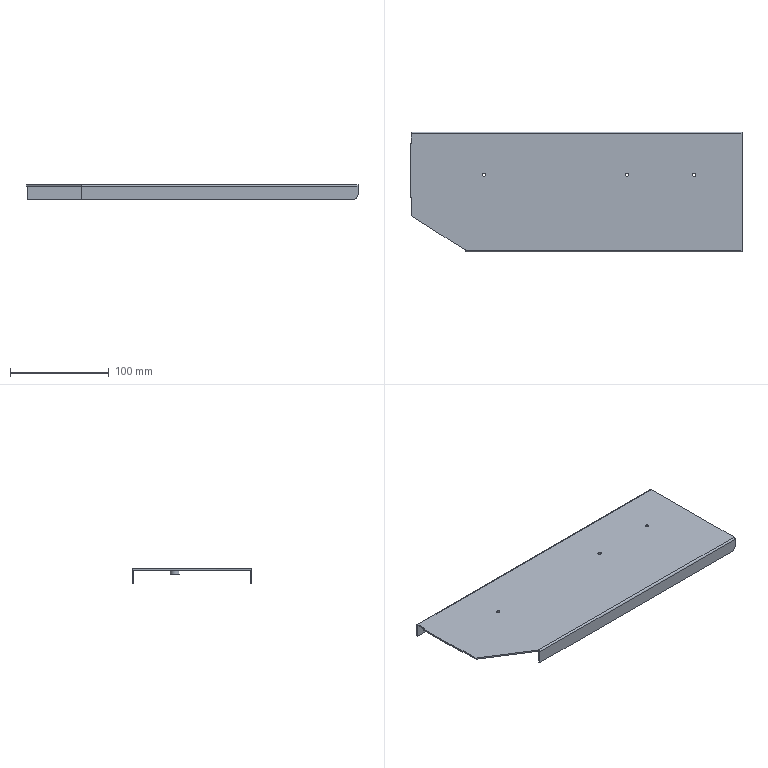Part | STEP file | FHD-021-001-U rack welded part U | 1 solid | 33 faces | box 336.5 x 121.5 x 15 mm | volume 72345 mm3 | plane 21 | cylinder 12 | commonest cylinder face diameters 3.3 x3 9.3 x3 0.4 x2 3.4 x2 10 x2